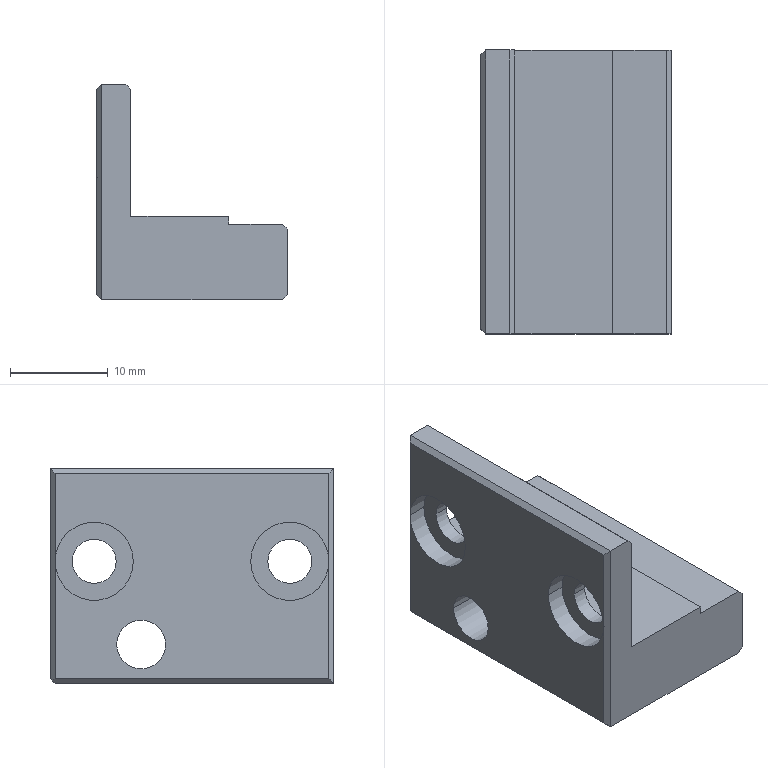Part | NX | 1 solid | 30 faces | box 19.5 x 29 x 22 mm | volume 5380 mm3 | plane 20 | cylinder 10 | commonest cylinder face diameters 4.5 x4 8 x4 5 x2
STEP:
#1=CARTESIAN_POINT('',(14.,3.2,-9.8));
#2=VERTEX_POINT('',#1);
#3=CARTESIAN_POINT('',(14.,32.2,-9.8));
#4=VERTEX_POINT('',#3);
#5=CARTESIAN_POINT('',(14.,0.,-9.8));
#6=DIRECTION('',(0.,1.,0.));
#7=VECTOR('',#6,1000.);
#8=LINE('',#5,#7);
#9=EDGE_CURVE('',#2,#4,#8,.T.);
#10=ORIENTED_EDGE('',*,*,#9,.F.);
#11=CARTESIAN_POINT('',(19.5,3.2,-9.8));
#12=VERTEX_POINT('',#11);
#13=CARTESIAN_POINT('',(0.,3.2,-9.8));
#14=DIRECTION('',(-1.,0.,0.));
#15=VECTOR('',#14,1000.);
#16=LINE('',#13,#15);
#17=EDGE_CURVE('',#12,#2,#16,.T.);
#18=ORIENTED_EDGE('',*,*,#17,.F.);
#19=CARTESIAN_POINT('',(19.5,32.2,-9.8));
#20=VERTEX_POINT('',#19);
#21=CARTESIAN_POINT('',(19.5,0.,-9.8));
#22=DIRECTION('',(0.,1.,0.));
#23=VECTOR('',#22,1000.);
#24=LINE('',#21,#23);
#25=EDGE_CURVE('',#12,#20,#24,.T.);
#26=ORIENTED_EDGE('',*,*,#25,.T.);
#27=CARTESIAN_POINT('',(0.,32.2,-9.8));
#28=DIRECTION('',(1.,0.,0.));
#29=VECTOR('',#28,1000.);
#30=LINE('',#27,#29);
#31=EDGE_CURVE('',#4,#20,#30,.T.);
#32=ORIENTED_EDGE('',*,*,#31,.F.);
#33=EDGE_LOOP('',(#10,#18,#26,#32));
#34=FACE_BOUND('',#33,.T.);
#35=CARTESIAN_POINT('',(14.,14.5,-9.8));
#36=DIRECTION('',(0.,0.,1.));
#37=DIRECTION('',(1.,0.,0.));
#38=AXIS2_PLACEMENT_3D('',#35,#36,#37);
#39=PLANE('',#38);
#40=ADVANCED_FACE('',(#34),#39,.T.);
#41=CARTESIAN_POINT('',(20.,32.2,-10.3));
#42=VERTEX_POINT('',#41);
#43=CARTESIAN_POINT('',(20.,3.2,-10.3));
#44=VERTEX_POINT('',#43);
#45=CARTESIAN_POINT('',(20.,0.,-10.3));
#46=DIRECTION('',(0.,-1.,0.));
#47=VECTOR('',#46,1000.);
#48=LINE('',#45,#47);
#49=EDGE_CURVE('',#42,#44,#48,.T.);
#50=ORIENTED_EDGE('',*,*,#49,.T.);
#51=CARTESIAN_POINT('',(20.,3.2,-17.));
#52=VERTEX_POINT('',#51);
#53=CARTESIAN_POINT('',(20.,3.2,0.));
#54=DIRECTION('',(0.,0.,1.));
#55=VECTOR('',#54,1000.);
#56=LINE('',#53,#55);
#57=EDGE_CURVE('',#52,#44,#56,.T.);
#58=ORIENTED_EDGE('',*,*,#57,.F.);
#59=CARTESIAN_POINT('',(20.,32.2,-17.));
#60=VERTEX_POINT('',#59);
#61=CARTESIAN_POINT('',(20.,0.,-17.));
#62=DIRECTION('',(0.,-1.,0.));
#63=VECTOR('',#62,1000.);
#64=LINE('',#61,#63);
#65=EDGE_CURVE('',#60,#52,#64,.T.);
#66=ORIENTED_EDGE('',*,*,#65,.F.);
#67=CARTESIAN_POINT('',(20.,32.2,0.));
#68=DIRECTION('',(0.,0.,1.));
#69=VECTOR('',#68,1000.);
#70=LINE('',#67,#69);
#71=EDGE_CURVE('',#60,#42,#70,.T.);
#72=ORIENTED_EDGE('',*,*,#71,.T.);
#73=EDGE_LOOP('',(#50,#58,#66,#72));
#74=FACE_BOUND('',#73,.T.);
#75=CARTESIAN_POINT('',(20.,25.4,-13.5));
#76=VERTEX_POINT('',#75);
#77=CARTESIAN_POINT('',(20.,20.4,-13.5));
#78=VERTEX_POINT('',#77);
#79=CARTESIAN_POINT('',(20.,22.9,-13.5));
#80=DIRECTION('',(1.,0.,0.));
#81=DIRECTION('',(0.,1.,0.));
#82=AXIS2_PLACEMENT_3D('',#79,#80,#81);
#83=CIRCLE('',#82,2.5);
#84=EDGE_CURVE('',#76,#78,#83,.T.);
#85=ORIENTED_EDGE('',*,*,#84,.F.);
#86=CARTESIAN_POINT('',(20.,22.9,-13.5));
#87=DIRECTION('',(1.,0.,0.));
#88=DIRECTION('',(0.,1.,0.));
#89=AXIS2_PLACEMENT_3D('',#86,#87,#88);
#90=CIRCLE('',#89,2.5);
#91=EDGE_CURVE('',#78,#76,#90,.T.);
#92=ORIENTED_EDGE('',*,*,#91,.F.);
#93=EDGE_LOOP('',(#85,#92));
#94=FACE_BOUND('',#93,.T.);
#95=CARTESIAN_POINT('',(20.,14.5,-10.3));
#96=DIRECTION('',(1.,0.,0.));
#97=DIRECTION('',(0.,1.,0.));
#98=AXIS2_PLACEMENT_3D('',#95,#96,#97);
#99=PLANE('',#98);
#100=ADVANCED_FACE('',(#74,#94),#99,.T.);
#101=CARTESIAN_POINT('',(1.,3.2,4.5));
#102=VERTEX_POINT('',#101);
#103=CARTESIAN_POINT('',(1.,3.2,-17.5));
#104=VERTEX_POINT('',#103);
#105=CARTESIAN_POINT('',(1.,3.2,0.));
#106=DIRECTION('',(0.,0.,-1.));
#107=VECTOR('',#106,1000.);
#108=LINE('',#105,#107);
#109=EDGE_CURVE('',#102,#104,#108,.T.);
#110=ORIENTED_EDGE('',*,*,#109,.F.);
#111=CARTESIAN_POINT('',(0.5,3.7,4.));
#112=VERTEX_POINT('',#111);
#113=CARTESIAN_POINT('',(-3.5,7.7,0.));
#114=DIRECTION('',(0.5774,-0.5774,0.5774));
#115=VECTOR('',#114,1000.);
#116=LINE('',#113,#115);
#117=EDGE_CURVE('',#112,#102,#116,.T.);
#118=ORIENTED_EDGE('',*,*,#117,.F.);
#119=CARTESIAN_POINT('',(0.5,3.7,-5.));
#120=VERTEX_POINT('',#119);
#121=CARTESIAN_POINT('',(0.5,3.7,0.));
#122=DIRECTION('',(0.,0.,1.));
#123=VECTOR('',#122,1000.);
#124=LINE('',#121,#123);
#125=EDGE_CURVE('',#120,#112,#124,.T.);
#126=ORIENTED_EDGE('',*,*,#125,.F.);
#127=CARTESIAN_POINT('',(0.5,3.7,-17.));
#128=VERTEX_POINT('',#127);
#129=CARTESIAN_POINT('',(0.5,3.7,0.));
#130=DIRECTION('',(0.,0.,1.));
#131=VECTOR('',#130,1000.);
#132=LINE('',#129,#131);
#133=EDGE_CURVE('',#128,#120,#132,.T.);
#134=ORIENTED_EDGE('',*,*,#133,.F.);
#135=CARTESIAN_POINT('',(-16.5,20.7,0.));
#136=DIRECTION('',(-0.5774,0.5774,0.5774));
#137=VECTOR('',#136,1000.);
#138=LINE('',#135,#137);
#139=EDGE_CURVE('',#104,#128,#138,.T.);
#140=ORIENTED_EDGE('',*,*,#139,.F.);
#141=EDGE_LOOP('',(#110,#118,#126,#134,#140));
#142=FACE_BOUND('',#141,.T.);
#143=CARTESIAN_POINT('',(0.75,3.45,-6.5));
#144=DIRECTION('',(0.7071,0.7071,0.));
#145=DIRECTION('',(0.,0.,-1.));
#146=AXIS2_PLACEMENT_3D('',#143,#144,#145);
#147=PLANE('',#146);
#148=ADVANCED_FACE('',(#142),#147,.F.);
#149=CARTESIAN_POINT('',(14.,32.2,-9.));
#150=VERTEX_POINT('',#149);
#151=CARTESIAN_POINT('',(14.,3.2,-9.));
#152=VERTEX_POINT('',#151);
#153=CARTESIAN_POINT('',(14.,0.,-9.));
#154=DIRECTION('',(0.,-1.,0.));
#155=VECTOR('',#154,1000.);
#156=LINE('',#153,#155);
#157=EDGE_CURVE('',#150,#152,#156,.T.);
#158=ORIENTED_EDGE('',*,*,#157,.F.);
#159=CARTESIAN_POINT('',(4.,32.2,-9.));
#160=VERTEX_POINT('',#159);
#161=CARTESIAN_POINT('',(0.,32.2,-9.));
#162=DIRECTION('',(-1.,0.,0.));
#163=VECTOR('',#162,1000.);
#164=LINE('',#161,#163);
#165=EDGE_CURVE('',#150,#160,#164,.T.);
#166=ORIENTED_EDGE('',*,*,#165,.T.);
#167=CARTESIAN_POINT('',(4.,3.2,-9.));
#168=VERTEX_POINT('',#167);
#169=CARTESIAN_POINT('',(4.,0.,-9.));
#170=DIRECTION('',(0.,1.,0.));
#171=VECTOR('',#170,1000.);
#172=LINE('',#169,#171);
#173=EDGE_CURVE('',#168,#160,#172,.T.);
#174=ORIENTED_EDGE('',*,*,#173,.F.);
#175=CARTESIAN_POINT('',(0.,3.2,-9.));
#176=DIRECTION('',(-1.,0.,0.));
#177=VECTOR('',#176,1000.);
#178=LINE('',#175,#177);
#179=EDGE_CURVE('',#152,#168,#178,.T.);
#180=ORIENTED_EDGE('',*,*,#179,.F.);
#181=EDGE_LOOP('',(#158,#166,#174,#180));
#182=FACE_BOUND('',#181,.T.);
#183=CARTESIAN_POINT('',(4.,0.,-9.));
#184=DIRECTION('',(0.,0.,1.));
#185=DIRECTION('',(1.,0.,0.));
#186=AXIS2_PLACEMENT_3D('',#183,#184,#185);
#187=PLANE('',#186);
#188=ADVANCED_FACE('',(#182),#187,.T.);
#189=ORIENTED_EDGE('',*,*,#109,.T.);
#190=CARTESIAN_POINT('',(19.5,3.2,-17.5));
#191=VERTEX_POINT('',#190);
#192=CARTESIAN_POINT('',(0.,3.2,-17.5));
#193=DIRECTION('',(1.,0.,0.));
#194=VECTOR('',#193,1000.);
#195=LINE('',#192,#194);
#196=EDGE_CURVE('',#104,#191,#195,.T.);
#197=ORIENTED_EDGE('',*,*,#196,.T.);
#198=CARTESIAN_POINT('',(37.,3.2,0.));
#199=DIRECTION('',(0.7071,0.,0.7071));
#200=VECTOR('',#199,1000.);
#201=LINE('',#198,#200);
#202=EDGE_CURVE('',#191,#52,#201,.T.);
#203=ORIENTED_EDGE('',*,*,#202,.T.);
#204=ORIENTED_EDGE('',*,*,#57,.T.);
#205=CARTESIAN_POINT('',(9.7,3.2,0.));
#206=DIRECTION('',(-0.7071,0.,0.7071));
#207=VECTOR('',#206,1000.);
#208=LINE('',#205,#207);
#209=EDGE_CURVE('',#44,#12,#208,.T.);
#210=ORIENTED_EDGE('',*,*,#209,.T.);
#211=ORIENTED_EDGE('',*,*,#17,.T.);
#212=CARTESIAN_POINT('',(14.,3.2,0.));
#213=DIRECTION('',(0.,0.,-1.));
#214=VECTOR('',#213,1000.);
#215=LINE('',#212,#214);
#216=EDGE_CURVE('',#152,#2,#215,.T.);
#217=ORIENTED_EDGE('',*,*,#216,.F.);
#218=ORIENTED_EDGE('',*,*,#179,.T.);
#219=CARTESIAN_POINT('',(4.,3.2,4.));
#220=VERTEX_POINT('',#219);
#221=CARTESIAN_POINT('',(4.,3.2,0.));
#222=DIRECTION('',(0.,0.,1.));
#223=VECTOR('',#222,1000.);
#224=LINE('',#221,#223);
#225=EDGE_CURVE('',#168,#220,#224,.T.);
#226=ORIENTED_EDGE('',*,*,#225,.T.);
#227=CARTESIAN_POINT('',(3.5,3.2,4.5));
#228=VERTEX_POINT('',#227);
#229=CARTESIAN_POINT('',(8.,3.2,0.));
#230=DIRECTION('',(0.7071,0.,-0.7071));
#231=VECTOR('',#230,1000.);
#232=LINE('',#229,#231);
#233=EDGE_CURVE('',#228,#220,#232,.T.);
#234=ORIENTED_EDGE('',*,*,#233,.F.);
#235=CARTESIAN_POINT('',(0.,3.2,4.5));
#236=DIRECTION('',(-1.,0.,0.));
#237=VECTOR('',#236,1000.);
#238=LINE('',#235,#237);
#239=EDGE_CURVE('',#228,#102,#238,.T.);
#240=ORIENTED_EDGE('',*,*,#239,.T.);
#241=EDGE_LOOP('',(#189,#197,#203,#204,#210,#211,#217,#218,#226,#234,#240));
#242=FACE_BOUND('',#241,.T.);
#243=CARTESIAN_POINT('',(17.967,3.2,-12.374));
#244=DIRECTION('',(0.,-1.,0.));
#245=DIRECTION('',(0.,0.,-1.));
#246=AXIS2_PLACEMENT_3D('',#243,#244,#245);
#247=PLANE('',#246);
#248=ADVANCED_FACE('',(#242),#247,.T.);
#249=CARTESIAN_POINT('',(1.,32.2,4.5));
#250=VERTEX_POINT('',#249);
#251=CARTESIAN_POINT('',(1.,0.,4.5));
#252=DIRECTION('',(0.,-1.,0.));
#253=VECTOR('',#252,1000.);
#254=LINE('',#251,#253);
#255=EDGE_CURVE('',#250,#102,#254,.T.);
#256=ORIENTED_EDGE('',*,*,#255,.T.);
#257=ORIENTED_EDGE('',*,*,#239,.F.);
#258=CARTESIAN_POINT('',(3.5,32.2,4.5));
#259=VERTEX_POINT('',#258);
#260=CARTESIAN_POINT('',(3.5,0.,4.5));
#261=DIRECTION('',(0.,-1.,0.));
#262=VECTOR('',#261,1000.);
#263=LINE('',#260,#262);
#264=EDGE_CURVE('',#259,#228,#263,.T.);
#265=ORIENTED_EDGE('',*,*,#264,.F.);
#266=CARTESIAN_POINT('',(0.,32.2,4.5));
#267=DIRECTION('',(-1.,0.,0.));
#268=VECTOR('',#267,1000.);
#269=LINE('',#266,#268);
#270=EDGE_CURVE('',#259,#250,#269,.T.);
#271=ORIENTED_EDGE('',*,*,#270,.T.);
#272=EDGE_LOOP('',(#256,#257,#265,#271));
#273=FACE_BOUND('',#272,.T.);
#274=CARTESIAN_POINT('',(0.,0.,4.5));
#275=DIRECTION('',(0.,0.,1.));
#276=DIRECTION('',(1.,0.,0.));
#277=AXIS2_PLACEMENT_3D('',#274,#275,#276);
#278=PLANE('',#277);
#279=ADVANCED_FACE('',(#273),#278,.T.);
#280=CARTESIAN_POINT('',(2.5,11.7,-5.));
#281=VERTEX_POINT('',#280);
#282=CARTESIAN_POINT('',(2.5,3.7,-5.));
#283=VERTEX_POINT('',#282);
#284=CARTESIAN_POINT('',(2.5,7.7,-5.));
#285=DIRECTION('',(-1.,0.,0.));
#286=DIRECTION('',(0.,1.,0.));
#287=AXIS2_PLACEMENT_3D('',#284,#285,#286);
#288=CIRCLE('',#287,4.);
#289=EDGE_CURVE('',#281,#283,#288,.T.);
#290=ORIENTED_EDGE('',*,*,#289,.T.);
#291=CARTESIAN_POINT('',(2.5,7.7,-5.));
#292=DIRECTION('',(-1.,0.,0.));
#293=DIRECTION('',(0.,1.,0.));
#294=AXIS2_PLACEMENT_3D('',#291,#292,#293);
#295=CIRCLE('',#294,4.);
#296=EDGE_CURVE('',#283,#281,#295,.T.);
#297=ORIENTED_EDGE('',*,*,#296,.T.);
#298=EDGE_LOOP('',(#290,#297));
#299=FACE_BOUND('',#298,.T.);
#300=CARTESIAN_POINT('',(2.5,5.45,-5.));
#301=VERTEX_POINT('',#300);
#302=CARTESIAN_POINT('',(2.5,9.95,-5.));
#303=VERTEX_POINT('',#302);
#304=CARTESIAN_POINT('',(2.5,7.7,-5.));
#305=DIRECTION('',(-1.,0.,0.));
#306=DIRECTION('',(0.,1.,0.));
#307=AXIS2_PLACEMENT_3D('',#304,#305,#306);
#308=CIRCLE('',#307,2.25);
#309=EDGE_CURVE('',#301,#303,#308,.T.);
#310=ORIENTED_EDGE('',*,*,#309,.F.);
#311=CARTESIAN_POINT('',(2.5,7.7,-5.));
#312=DIRECTION('',(-1.,0.,0.));
#313=DIRECTION('',(0.,1.,0.));
#314=AXIS2_PLACEMENT_3D('',#311,#312,#313);
#315=CIRCLE('',#314,2.25);
#316=EDGE_CURVE('',#303,#301,#315,.T.);
#317=ORIENTED_EDGE('',*,*,#316,.F.);
#318=EDGE_LOOP('',(#310,#317));
#319=FACE_BOUND('',#318,.T.);
#320=CARTESIAN_POINT('',(2.5,7.7,-5.));
#321=DIRECTION('',(-1.,0.,0.));
#322=DIRECTION('',(0.,0.,1.));
#323=AXIS2_PLACEMENT_3D('',#320,#321,#322);
#324=PLANE('',#323);
#325=ADVANCED_FACE('',(#299,#319),#324,.T.);
#326=CARTESIAN_POINT('',(1.,32.2,-17.));
#327=VERTEX_POINT('',#326);
#328=CARTESIAN_POINT('',(0.,32.2,-17.));
#329=DIRECTION('',(-1.,0.,0.));
#330=VECTOR('',#329,1000.);
#331=LINE('',#328,#330);
#332=EDGE_CURVE('',#60,#327,#331,.T.);
#333=ORIENTED_EDGE('',*,*,#332,.T.);
#334=CARTESIAN_POINT('',(1.,32.2,0.));
#335=DIRECTION('',(0.,0.,-1.));
#336=VECTOR('',#335,1000.);
#337=LINE('',#334,#336);
#338=EDGE_CURVE('',#250,#327,#337,.T.);
#339=ORIENTED_EDGE('',*,*,#338,.F.);
#340=ORIENTED_EDGE('',*,*,#270,.F.);
#341=CARTESIAN_POINT('',(4.,32.2,4.));
#342=VERTEX_POINT('',#341);
#343=CARTESIAN_POINT('',(8.,32.2,0.));
#344=DIRECTION('',(0.7071,0.,-0.7071));
#345=VECTOR('',#344,1000.);
#346=LINE('',#343,#345);
#347=EDGE_CURVE('',#259,#342,#346,.T.);
#348=ORIENTED_EDGE('',*,*,#347,.T.);
#349=CARTESIAN_POINT('',(4.,32.2,0.));
#350=DIRECTION('',(0.,0.,-1.));
#351=VECTOR('',#350,1000.);
#352=LINE('',#349,#351);
#353=EDGE_CURVE('',#342,#160,#352,.T.);
#354=ORIENTED_EDGE('',*,*,#353,.T.);
#355=ORIENTED_EDGE('',*,*,#165,.F.);
#356=CARTESIAN_POINT('',(14.,32.2,0.));
#357=DIRECTION('',(0.,0.,-1.));
#358=VECTOR('',#357,1000.);
#359=LINE('',#356,#358);
#360=EDGE_CURVE('',#150,#4,#359,.T.);
#361=ORIENTED_EDGE('',*,*,#360,.T.);
#362=ORIENTED_EDGE('',*,*,#31,.T.);
#363=CARTESIAN_POINT('',(9.7,32.2,0.));
#364=DIRECTION('',(0.7071,0.,-0.7071));
#365=VECTOR('',#364,1000.);
#366=LINE('',#363,#365);
#367=EDGE_CURVE('',#20,#42,#366,.T.);
#368=ORIENTED_EDGE('',*,*,#367,.T.);
#369=ORIENTED_EDGE('',*,*,#71,.F.);
#370=EDGE_LOOP('',(#333,#339,#340,#348,#354,#355,#361,#362,#368,#369));
#371=FACE_BOUND('',#370,.T.);
#372=CARTESIAN_POINT('',(0.,32.2,0.));
#373=DIRECTION('',(0.,1.,0.));
#374=DIRECTION('',(1.,0.,0.));
#375=AXIS2_PLACEMENT_3D('',#372,#373,#374);
#376=PLANE('',#375);
#377=ADVANCED_FACE('',(#371),#376,.T.);
#378=CARTESIAN_POINT('',(0.5,31.7,4.));
#379=VERTEX_POINT('',#378);
#380=CARTESIAN_POINT('',(0.5,0.,4.));
#381=DIRECTION('',(0.,-1.,0.));
#382=VECTOR('',#381,1000.);
#383=LINE('',#380,#382);
#384=EDGE_CURVE('',#379,#112,#383,.T.);
#385=ORIENTED_EDGE('',*,*,#384,.F.);
#386=CARTESIAN_POINT('',(0.5,31.7,-5.));
#387=VERTEX_POINT('',#386);
#388=CARTESIAN_POINT('',(0.5,31.7,0.));
#389=DIRECTION('',(0.,0.,1.));
#390=VECTOR('',#389,1000.);
#391=LINE('',#388,#390);
#392=EDGE_CURVE('',#387,#379,#391,.T.);
#393=ORIENTED_EDGE('',*,*,#392,.F.);
#394=CARTESIAN_POINT('',(0.5,23.7,-5.));
#395=VERTEX_POINT('',#394);
#396=CARTESIAN_POINT('',(0.5,27.7,-5.));
#397=DIRECTION('',(-1.,0.,0.));
#398=DIRECTION('',(0.,1.,0.));
#399=AXIS2_PLACEMENT_3D('',#396,#397,#398);
#400=CIRCLE('',#399,4.);
#401=EDGE_CURVE('',#395,#387,#400,.T.);
#402=ORIENTED_EDGE('',*,*,#401,.F.);
#403=CARTESIAN_POINT('',(0.5,27.7,-5.));
#404=DIRECTION('',(-1.,0.,0.));
#405=DIRECTION('',(0.,1.,0.));
#406=AXIS2_PLACEMENT_3D('',#403,#404,#405);
#407=CIRCLE('',#406,4.);
#408=EDGE_CURVE('',#387,#395,#407,.T.);
#409=ORIENTED_EDGE('',*,*,#408,.F.);
#410=CARTESIAN_POINT('',(0.5,31.7,-17.));
#411=VERTEX_POINT('',#410);
#412=CARTESIAN_POINT('',(0.5,31.7,0.));
#413=DIRECTION('',(0.,0.,1.));
#414=VECTOR('',#413,1000.);
#415=LINE('',#412,#414);
#416=EDGE_CURVE('',#411,#387,#415,.T.);
#417=ORIENTED_EDGE('',*,*,#416,.F.);
#418=CARTESIAN_POINT('',(0.5,0.,-17.));
#419=DIRECTION('',(0.,1.,0.));
#420=VECTOR('',#419,1000.);
#421=LINE('',#418,#420);
#422=EDGE_CURVE('',#128,#411,#421,.T.);
#423=ORIENTED_EDGE('',*,*,#422,.F.);
#424=ORIENTED_EDGE('',*,*,#133,.T.);
#425=CARTESIAN_POINT('',(0.5,11.7,-5.));
#426=VERTEX_POINT('',#425);
#427=CARTESIAN_POINT('',(0.5,7.7,-5.));
#428=DIRECTION('',(-1.,0.,0.));
#429=DIRECTION('',(0.,1.,0.));
#430=AXIS2_PLACEMENT_3D('',#427,#428,#429);
#431=CIRCLE('',#430,4.);
#432=EDGE_CURVE('',#426,#120,#431,.T.);
#433=ORIENTED_EDGE('',*,*,#432,.F.);
#434=CARTESIAN_POINT('',(0.5,7.7,-5.));
#435=DIRECTION('',(-1.,0.,0.));
#436=DIRECTION('',(0.,1.,0.));
#437=AXIS2_PLACEMENT_3D('',#434,#435,#436);
#438=CIRCLE('',#437,4.);
#439=EDGE_CURVE('',#120,#426,#438,.T.);
#440=ORIENTED_EDGE('',*,*,#439,.F.);
#441=ORIENTED_EDGE('',*,*,#125,.T.);
#442=EDGE_LOOP('',(#385,#393,#402,#409,#417,#423,#424,#433,#440,#441));
#443=FACE_BOUND('',#442,.T.);
#444=CARTESIAN_POINT('',(0.5,25.4,-13.5));
#445=VERTEX_POINT('',#444);
#446=CARTESIAN_POINT('',(0.5,20.4,-13.5));
#447=VERTEX_POINT('',#446);
#448=CARTESIAN_POINT('',(0.5,22.9,-13.5));
#449=DIRECTION('',(1.,0.,0.));
#450=DIRECTION('',(0.,1.,0.));
#451=AXIS2_PLACEMENT_3D('',#448,#449,#450);
#452=CIRCLE('',#451,2.5);
#453=EDGE_CURVE('',#445,#447,#452,.T.);
#454=ORIENTED_EDGE('',*,*,#453,.T.);
#455=CARTESIAN_POINT('',(0.5,22.9,-13.5));
#456=DIRECTION('',(1.,0.,0.));
#457=DIRECTION('',(0.,1.,0.));
#458=AXIS2_PLACEMENT_3D('',#455,#456,#457);
#459=CIRCLE('',#458,2.5);
#460=EDGE_CURVE('',#447,#445,#459,.T.);
#461=ORIENTED_EDGE('',*,*,#460,.T.);
#462=EDGE_LOOP('',(#454,#461));
#463=FACE_BOUND('',#462,.T.);
#464=CARTESIAN_POINT('',(0.5,14.5,-17.));
#465=DIRECTION('',(-1.,0.,0.));
#466=DIRECTION('',(0.,0.,1.));
#467=AXIS2_PLACEMENT_3D('',#464,#465,#466);
#468=PLANE('',#467);
#469=ADVANCED_FACE('',(#443,#463),#468,.T.);
#470=ORIENTED_EDGE('',*,*,#117,.T.);
#471=ORIENTED_EDGE('',*,*,#255,.F.);
#472=CARTESIAN_POINT('',(-3.5,27.7,0.));
#473=DIRECTION('',(0.5774,0.5774,0.5774));
#474=VECTOR('',#473,1000.);
#475=LINE('',#472,#474);
#476=EDGE_CURVE('',#379,#250,#475,.T.);
#477=ORIENTED_EDGE('',*,*,#476,.F.);
#478=ORIENTED_EDGE('',*,*,#384,.T.);
#479=EDGE_LOOP('',(#470,#471,#477,#478));
#480=FACE_BOUND('',#479,.T.);
#481=CARTESIAN_POINT('',(0.75,17.,4.25));
#482=DIRECTION('',(-0.7071,0.,0.7071));
#483=DIRECTION('',(0.,1.,0.));
#484=AXIS2_PLACEMENT_3D('',#481,#482,#483);
#485=PLANE('',#484);
#486=ADVANCED_FACE('',(#480),#485,.T.);
#487=ORIENTED_EDGE('',*,*,#453,.F.);
#488=CARTESIAN_POINT('',(0.,25.4,-13.5));
#489=DIRECTION('',(1.,0.,0.));
#490=VECTOR('',#489,1000.);
#491=LINE('',#488,#490);
#492=EDGE_CURVE('',#445,#76,#491,.T.);
#493=ORIENTED_EDGE('',*,*,#492,.T.);
#494=ORIENTED_EDGE('',*,*,#84,.T.);
#495=CARTESIAN_POINT('',(0.,20.4,-13.5));
#496=DIRECTION('',(1.,0.,0.));
#497=VECTOR('',#496,1000.);
#498=LINE('',#495,#497);
#499=EDGE_CURVE('',#447,#78,#498,.T.);
#500=ORIENTED_EDGE('',*,*,#499,.F.);
#501=EDGE_LOOP('',(#487,#493,#494,#500));
#502=FACE_BOUND('',#501,.T.);
#503=CARTESIAN_POINT('',(0.,22.9,-13.5));
#504=DIRECTION('',(1.,0.,0.));
#505=DIRECTION('',(0.,1.,0.));
#506=AXIS2_PLACEMENT_3D('',#503,#504,#505);
#507=CYLINDRICAL_SURFACE('',#506,2.5);
#508=ADVANCED_FACE('',(#502),#507,.F.);
#509=CARTESIAN_POINT('',(2.5,31.7,-5.));
#510=VERTEX_POINT('',#509);
#511=CARTESIAN_POINT('',(2.5,23.7,-5.));
#512=VERTEX_POINT('',#511);
#513=CARTESIAN_POINT('',(2.5,27.7,-5.));
#514=DIRECTION('',(-1.,0.,0.));
#515=DIRECTION('',(0.,1.,0.));
#516=AXIS2_PLACEMENT_3D('',#513,#514,#515);
#517=CIRCLE('',#516,4.);
#518=EDGE_CURVE('',#510,#512,#517,.T.);
#519=ORIENTED_EDGE('',*,*,#518,.T.);
#520=CARTESIAN_POINT('',(2.5,27.7,-5.));
#521=DIRECTION('',(-1.,0.,0.));
#522=DIRECTION('',(0.,1.,0.));
#523=AXIS2_PLACEMENT_3D('',#520,#521,#522);
#524=CIRCLE('',#523,4.);
#525=EDGE_CURVE('',#512,#510,#524,.T.);
#526=ORIENTED_EDGE('',*,*,#525,.T.);
#527=EDGE_LOOP('',(#519,#526));
#528=FACE_BOUND('',#527,.T.);
#529=CARTESIAN_POINT('',(2.5,29.95,-5.));
#530=VERTEX_POINT('',#529);
#531=CARTESIAN_POINT('',(2.5,25.45,-5.));
#532=VERTEX_POINT('',#531);
#533=CARTESIAN_POINT('',(2.5,27.7,-5.));
#534=DIRECTION('',(-1.,0.,0.));
#535=DIRECTION('',(0.,1.,0.));
#536=AXIS2_PLACEMENT_3D('',#533,#534,#535);
#537=CIRCLE('',#536,2.25);
#538=EDGE_CURVE('',#530,#532,#537,.T.);
#539=ORIENTED_EDGE('',*,*,#538,.F.);
#540=CARTESIAN_POINT('',(2.5,27.7,-5.));
#541=DIRECTION('',(-1.,0.,0.));
#542=DIRECTION('',(0.,1.,0.));
#543=AXIS2_PLACEMENT_3D('',#540,#541,#542);
#544=CIRCLE('',#543,2.25);
#545=EDGE_CURVE('',#532,#530,#544,.T.);
#546=ORIENTED_EDGE('',*,*,#545,.F.);
#547=EDGE_LOOP('',(#539,#546));
#548=FACE_BOUND('',#547,.T.);
#549=CARTESIAN_POINT('',(2.5,27.7,-5.));
#550=DIRECTION('',(-1.,0.,0.));
#551=DIRECTION('',(0.,0.,1.));
#552=AXIS2_PLACEMENT_3D('',#549,#550,#551);
#553=PLANE('',#552);
#554=ADVANCED_FACE('',(#528,#548),#553,.T.);
#555=ORIENTED_EDGE('',*,*,#432,.T.);
#556=CARTESIAN_POINT('',(23.1,3.7,-5.));
#557=DIRECTION('',(-1.,0.,0.));
#558=VECTOR('',#557,1000.);
#559=LINE('',#556,#558);
#560=EDGE_CURVE('',#283,#120,#559,.T.);
#561=ORIENTED_EDGE('',*,*,#560,.F.);
#562=ORIENTED_EDGE('',*,*,#289,.F.);
#563=CARTESIAN_POINT('',(23.1,11.7,-5.));
#564=DIRECTION('',(-1.,0.,0.));
#565=VECTOR('',#564,1000.);
#566=LINE('',#563,#565);
#567=EDGE_CURVE('',#281,#426,#566,.T.);
#568=ORIENTED_EDGE('',*,*,#567,.T.);
#569=EDGE_LOOP('',(#555,#561,#562,#568));
#570=FACE_BOUND('',#569,.T.);
#571=CARTESIAN_POINT('',(23.1,7.7,-5.));
#572=DIRECTION('',(-1.,0.,0.));
#573=DIRECTION('',(0.,1.,0.));
#574=AXIS2_PLACEMENT_3D('',#571,#572,#573);
#575=CYLINDRICAL_SURFACE('',#574,4.);
#576=ADVANCED_FACE('',(#570),#575,.F.);
#577=ORIENTED_EDGE('',*,*,#538,.T.);
#578=CARTESIAN_POINT('',(4.,25.45,-5.));
#579=VERTEX_POINT('',#578);
#580=CARTESIAN_POINT('',(23.1,25.45,-5.));
#581=DIRECTION('',(-1.,0.,0.));
#582=VECTOR('',#581,1000.);
#583=LINE('',#580,#582);
#584=EDGE_CURVE('',#579,#532,#583,.T.);
#585=ORIENTED_EDGE('',*,*,#584,.F.);
#586=CARTESIAN_POINT('',(4.,29.95,-5.));
#587=VERTEX_POINT('',#586);
#588=CARTESIAN_POINT('',(4.,27.7,-5.));
#589=DIRECTION('',(-1.,0.,0.));
#590=DIRECTION('',(0.,1.,0.));
#591=AXIS2_PLACEMENT_3D('',#588,#589,#590);
#592=CIRCLE('',#591,2.25);
#593=EDGE_CURVE('',#587,#579,#592,.T.);
#594=ORIENTED_EDGE('',*,*,#593,.F.);
#595=CARTESIAN_POINT('',(23.1,29.95,-5.));
#596=DIRECTION('',(-1.,0.,0.));
#597=VECTOR('',#596,1000.);
#598=LINE('',#595,#597);
#599=EDGE_CURVE('',#587,#530,#598,.T.);
#600=ORIENTED_EDGE('',*,*,#599,.T.);
#601=EDGE_LOOP('',(#577,#585,#594,#600));
#602=FACE_BOUND('',#601,.T.);
#603=CARTESIAN_POINT('',(23.1,27.7,-5.));
#604=DIRECTION('',(-1.,0.,0.));
#605=DIRECTION('',(0.,1.,0.));
#606=AXIS2_PLACEMENT_3D('',#603,#604,#605);
#607=CYLINDRICAL_SURFACE('',#606,2.25);
#608=ADVANCED_FACE('',(#602),#607,.F.);
#609=CARTESIAN_POINT('',(4.,0.,4.));
#610=DIRECTION('',(0.,-1.,0.));
#611=VECTOR('',#610,1000.);
#612=LINE('',#609,#611);
#613=EDGE_CURVE('',#342,#220,#612,.T.);
#614=ORIENTED_EDGE('',*,*,#613,.T.);
#615=ORIENTED_EDGE('',*,*,#225,.F.);
#616=ORIENTED_EDGE('',*,*,#173,.T.);
#617=ORIENTED_EDGE('',*,*,#353,.F.);
#618=EDGE_LOOP('',(#614,#615,#616,#617));
#619=FACE_BOUND('',#618,.T.);
#620=CARTESIAN_POINT('',(4.,9.95,-5.));
#621=VERTEX_POINT('',#620);
#622=CARTESIAN_POINT('',(4.,5.45,-5.));
#623=VERTEX_POINT('',#622);
#624=CARTESIAN_POINT('',(4.,7.7,-5.));
#625=DIRECTION('',(-1.,0.,0.));
#626=DIRECTION('',(0.,1.,0.));
#627=AXIS2_PLACEMENT_3D('',#624,#625,#626);
#628=CIRCLE('',#627,2.25);
#629=EDGE_CURVE('',#621,#623,#628,.T.);
#630=ORIENTED_EDGE('',*,*,#629,.T.);
#631=CARTESIAN_POINT('',(4.,7.7,-5.));
#632=DIRECTION('',(-1.,0.,0.));
#633=DIRECTION('',(0.,1.,0.));
#634=AXIS2_PLACEMENT_3D('',#631,#632,#633);
#635=CIRCLE('',#634,2.25);
#636=EDGE_CURVE('',#623,#621,#635,.T.);
#637=ORIENTED_EDGE('',*,*,#636,.T.);
#638=EDGE_LOOP('',(#630,#637));
#639=FACE_BOUND('',#638,.T.);
#640=ORIENTED_EDGE('',*,*,#593,.T.);
#641=CARTESIAN_POINT('',(4.,27.7,-5.));
#642=DIRECTION('',(-1.,0.,0.));
#643=DIRECTION('',(0.,1.,0.));
#644=AXIS2_PLACEMENT_3D('',#641,#642,#643);
#645=CIRCLE('',#644,2.25);
#646=EDGE_CURVE('',#579,#587,#645,.T.);
#647=ORIENTED_EDGE('',*,*,#646,.T.);
#648=EDGE_LOOP('',(#640,#647));
#649=FACE_BOUND('',#648,.T.);
#650=CARTESIAN_POINT('',(4.,0.,0.));
#651=DIRECTION('',(1.,0.,0.));
#652=DIRECTION('',(0.,1.,0.));
#653=AXIS2_PLACEMENT_3D('',#650,#651,#652);
#654=PLANE('',#653);
#655=ADVANCED_FACE('',(#619,#639,#649),#654,.T.);
#656=ORIENTED_EDGE('',*,*,#629,.F.);
#657=CARTESIAN_POINT('',(23.1,9.95,-5.));
#658=DIRECTION('',(-1.,0.,0.));
#659=VECTOR('',#658,1000.);
#660=LINE('',#657,#659);
#661=EDGE_CURVE('',#621,#303,#660,.T.);
#662=ORIENTED_EDGE('',*,*,#661,.T.);
#663=ORIENTED_EDGE('',*,*,#316,.T.);
#664=CARTESIAN_POINT('',(23.1,5.45,-5.));
#665=DIRECTION('',(-1.,0.,0.));
#666=VECTOR('',#665,1000.);
#667=LINE('',#664,#666);
#668=EDGE_CURVE('',#623,#301,#667,.T.);
#669=ORIENTED_EDGE('',*,*,#668,.F.);
#670=EDGE_LOOP('',(#656,#662,#663,#669));
#671=FACE_BOUND('',#670,.T.);
#672=CARTESIAN_POINT('',(23.1,7.7,-5.));
#673=DIRECTION('',(-1.,0.,0.));
#674=DIRECTION('',(0.,1.,0.));
#675=AXIS2_PLACEMENT_3D('',#672,#673,#674);
#676=CYLINDRICAL_SURFACE('',#675,2.25);
#677=ADVANCED_FACE('',(#671),#676,.F.);
#678=ORIENTED_EDGE('',*,*,#518,.F.);
#679=CARTESIAN_POINT('',(23.1,31.7,-5.));
#680=DIRECTION('',(-1.,0.,0.));
#681=VECTOR('',#680,1000.);
#682=LINE('',#679,#681);
#683=EDGE_CURVE('',#510,#387,#682,.T.);
#684=ORIENTED_EDGE('',*,*,#683,.T.);
#685=ORIENTED_EDGE('',*,*,#408,.T.);
#686=CARTESIAN_POINT('',(23.1,23.7,-5.));
#687=DIRECTION('',(-1.,0.,0.));
#688=VECTOR('',#687,1000.);
#689=LINE('',#686,#688);
#690=EDGE_CURVE('',#512,#395,#689,.T.);
#691=ORIENTED_EDGE('',*,*,#690,.F.);
#692=EDGE_LOOP('',(#678,#684,#685,#691));
#693=FACE_BOUND('',#692,.T.);
#694=CARTESIAN_POINT('',(23.1,27.7,-5.));
#695=DIRECTION('',(-1.,0.,0.));
#696=DIRECTION('',(0.,1.,0.));
#697=AXIS2_PLACEMENT_3D('',#694,#695,#696);
#698=CYLINDRICAL_SURFACE('',#697,4.);
#699=ADVANCED_FACE('',(#693),#698,.F.);
#700=CARTESIAN_POINT('',(19.5,31.7,-17.5));
#701=VERTEX_POINT('',#700);
#702=CARTESIAN_POINT('',(37.,49.2,0.));
#703=DIRECTION('',(0.5774,0.5774,0.5774));
#704=VECTOR('',#703,1000.);
#705=LINE('',#702,#704);
#706=EDGE_CURVE('',#701,#60,#705,.T.);
#707=ORIENTED_EDGE('',*,*,#706,.T.);
#708=ORIENTED_EDGE('',*,*,#65,.T.);
#709=ORIENTED_EDGE('',*,*,#202,.F.);
#710=CARTESIAN_POINT('',(19.5,0.,-17.5));
#711=DIRECTION('',(0.,1.,0.));
#712=VECTOR('',#711,1000.);
#713=LINE('',#710,#712);
#714=EDGE_CURVE('',#191,#701,#713,.T.);
#715=ORIENTED_EDGE('',*,*,#714,.T.);
#716=EDGE_LOOP('',(#707,#708,#709,#715));
#717=FACE_BOUND('',#716,.T.);
#718=CARTESIAN_POINT('',(20.,14.5,-17.));
#719=DIRECTION('',(0.7071,0.,-0.7071));
#720=DIRECTION('',(0.,-1.,0.));
#721=AXIS2_PLACEMENT_3D('',#718,#719,#720);
#722=PLANE('',#721);
#723=ADVANCED_FACE('',(#717),#722,.T.);
#724=CARTESIAN_POINT('',(1.,31.7,-17.5));
#725=VERTEX_POINT('',#724);
#726=CARTESIAN_POINT('',(1.,0.,-17.5));
#727=DIRECTION('',(0.,1.,0.));
#728=VECTOR('',#727,1000.);
#729=LINE('',#726,#728);
#730=EDGE_CURVE('',#104,#725,#729,.T.);
#731=ORIENTED_EDGE('',*,*,#730,.F.);
#732=ORIENTED_EDGE('',*,*,#139,.T.);
#733=ORIENTED_EDGE('',*,*,#422,.T.);
#734=CARTESIAN_POINT('',(0.75,31.95,-17.25));
#735=VERTEX_POINT('',#734);
#736=CARTESIAN_POINT('',(-16.5,14.7,0.));
#737=DIRECTION('',(-0.5774,-0.5774,0.5774));
#738=VECTOR('',#737,1000.);
#739=LINE('',#736,#738);
#740=EDGE_CURVE('',#735,#411,#739,.T.);
#741=ORIENTED_EDGE('',*,*,#740,.F.);
#742=CARTESIAN_POINT('',(-16.5,49.2,0.));
#743=DIRECTION('',(0.5774,-0.5774,-0.5774));
#744=VECTOR('',#743,1000.);
#745=LINE('',#742,#744);
#746=EDGE_CURVE('',#735,#725,#745,.T.);
#747=ORIENTED_EDGE('',*,*,#746,.T.);
#748=EDGE_LOOP('',(#731,#732,#733,#741,#747));
#749=FACE_BOUND('',#748,.T.);
#750=CARTESIAN_POINT('',(1.,14.5,-17.5));
#751=DIRECTION('',(-0.7071,0.,-0.7071));
#752=DIRECTION('',(-0.7071,0.,0.7071));
#753=AXIS2_PLACEMENT_3D('',#750,#751,#752);
#754=PLANE('',#753);
#755=ADVANCED_FACE('',(#749),#754,.T.);
#756=ORIENTED_EDGE('',*,*,#338,.T.);
#757=CARTESIAN_POINT('',(18.,49.2,0.));
#758=DIRECTION('',(-0.5774,-0.5774,-0.5774));
#759=VECTOR('',#758,1000.);
#760=LINE('',#757,#759);
#761=EDGE_CURVE('',#327,#735,#760,.T.);
#762=ORIENTED_EDGE('',*,*,#761,.T.);
#763=ORIENTED_EDGE('',*,*,#740,.T.);
#764=ORIENTED_EDGE('',*,*,#416,.T.);
#765=ORIENTED_EDGE('',*,*,#392,.T.);
#766=ORIENTED_EDGE('',*,*,#476,.T.);
#767=EDGE_LOOP('',(#756,#762,#763,#764,#765,#766));
#768=FACE_BOUND('',#767,.T.);
#769=CARTESIAN_POINT('',(0.75,31.95,-8.5));
#770=DIRECTION('',(-0.7071,0.7071,0.));
#771=DIRECTION('',(0.,0.,1.));
#772=AXIS2_PLACEMENT_3D('',#769,#770,#771);
#773=PLANE('',#772);
#774=ADVANCED_FACE('',(#768),#773,.T.);
#775=ORIENTED_EDGE('',*,*,#9,.T.);
#776=ORIENTED_EDGE('',*,*,#360,.F.);
#777=ORIENTED_EDGE('',*,*,#157,.T.);
#778=ORIENTED_EDGE('',*,*,#216,.T.);
#779=EDGE_LOOP('',(#775,#776,#777,#778));
#780=FACE_BOUND('',#779,.T.);
#781=CARTESIAN_POINT('',(14.,26.,-19.25));
#782=DIRECTION('',(-1.,0.,0.));
#783=DIRECTION('',(0.,0.,1.));
#784=AXIS2_PLACEMENT_3D('',#781,#782,#783);
#785=PLANE('',#784);
#786=ADVANCED_FACE('',(#780),#785,.F.);
#787=ORIENTED_EDGE('',*,*,#613,.F.);
#788=ORIENTED_EDGE('',*,*,#347,.F.);
#789=ORIENTED_EDGE('',*,*,#264,.T.);
#790=ORIENTED_EDGE('',*,*,#233,.T.);
#791=EDGE_LOOP('',(#787,#788,#789,#790));
#792=FACE_BOUND('',#791,.T.);
#793=CARTESIAN_POINT('',(3.75,17.,4.25));
#794=DIRECTION('',(-0.7071,0.,-0.7071));
#795=DIRECTION('',(-0.7071,0.,0.7071));
#796=AXIS2_PLACEMENT_3D('',#793,#794,#795);
#797=PLANE('',#796);
#798=ADVANCED_FACE('',(#792),#797,.F.);
#799=ORIENTED_EDGE('',*,*,#25,.F.);
#800=ORIENTED_EDGE('',*,*,#209,.F.);
#801=ORIENTED_EDGE('',*,*,#49,.F.);
#802=ORIENTED_EDGE('',*,*,#367,.F.);
#803=EDGE_LOOP('',(#799,#800,#801,#802));
#804=FACE_BOUND('',#803,.T.);
#805=CARTESIAN_POINT('',(19.75,19.25,-10.05));
#806=DIRECTION('',(0.7071,0.,0.7071));
#807=DIRECTION('',(0.,-1.,0.));
#808=AXIS2_PLACEMENT_3D('',#805,#806,#807);
#809=PLANE('',#808);
#810=ADVANCED_FACE('',(#804),#809,.T.);
#811=ORIENTED_EDGE('',*,*,#714,.F.);
#812=ORIENTED_EDGE('',*,*,#196,.F.);
#813=ORIENTED_EDGE('',*,*,#730,.T.);
#814=CARTESIAN_POINT('',(0.,31.7,-17.5));
#815=DIRECTION('',(1.,0.,0.));
#816=VECTOR('',#815,1000.);
#817=LINE('',#814,#816);
#818=EDGE_CURVE('',#725,#701,#817,.T.);
#819=ORIENTED_EDGE('',*,*,#818,.T.);
#820=EDGE_LOOP('',(#811,#812,#813,#819));
#821=FACE_BOUND('',#820,.T.);
#822=CARTESIAN_POINT('',(19.5,14.5,-17.5));
#823=DIRECTION('',(0.,0.,-1.));
#824=DIRECTION('',(0.,-1.,0.));
#825=AXIS2_PLACEMENT_3D('',#822,#823,#824);
#826=PLANE('',#825);
#827=ADVANCED_FACE('',(#821),#826,.T.);
#828=ORIENTED_EDGE('',*,*,#332,.F.);
#829=ORIENTED_EDGE('',*,*,#706,.F.);
#830=ORIENTED_EDGE('',*,*,#818,.F.);
#831=ORIENTED_EDGE('',*,*,#746,.F.);
#832=ORIENTED_EDGE('',*,*,#761,.F.);
#833=EDGE_LOOP('',(#828,#829,#830,#831,#832));
#834=FACE_BOUND('',#833,.T.);
#835=CARTESIAN_POINT('',(10.25,31.95,-17.25));
#836=DIRECTION('',(0.,-0.7071,0.7071));
#837=DIRECTION('',(-1.,0.,0.));
#838=AXIS2_PLACEMENT_3D('',#835,#836,#837);
#839=PLANE('',#838);
#840=ADVANCED_FACE('',(#834),#839,.F.);
#841=ORIENTED_EDGE('',*,*,#401,.T.);
#842=ORIENTED_EDGE('',*,*,#683,.F.);
#843=ORIENTED_EDGE('',*,*,#525,.F.);
#844=ORIENTED_EDGE('',*,*,#690,.T.);
#845=EDGE_LOOP('',(#841,#842,#843,#844));
#846=FACE_BOUND('',#845,.T.);
#847=CARTESIAN_POINT('',(23.1,27.7,-5.));
#848=DIRECTION('',(-1.,0.,0.));
#849=DIRECTION('',(0.,1.,0.));
#850=AXIS2_PLACEMENT_3D('',#847,#848,#849);
#851=CYLINDRICAL_SURFACE('',#850,4.);
#852=ADVANCED_FACE('',(#846),#851,.F.);
#853=ORIENTED_EDGE('',*,*,#309,.T.);
#854=ORIENTED_EDGE('',*,*,#661,.F.);
#855=ORIENTED_EDGE('',*,*,#636,.F.);
#856=ORIENTED_EDGE('',*,*,#668,.T.);
#857=EDGE_LOOP('',(#853,#854,#855,#856));
#858=FACE_BOUND('',#857,.T.);
#859=CARTESIAN_POINT('',(23.1,7.7,-5.));
#860=DIRECTION('',(-1.,0.,0.));
#861=DIRECTION('',(0.,1.,0.));
#862=AXIS2_PLACEMENT_3D('',#859,#860,#861);
#863=CYLINDRICAL_SURFACE('',#862,2.25);
#864=ADVANCED_FACE('',(#858),#863,.F.);
#865=ORIENTED_EDGE('',*,*,#492,.F.);
#866=ORIENTED_EDGE('',*,*,#460,.F.);
#867=ORIENTED_EDGE('',*,*,#499,.T.);
#868=ORIENTED_EDGE('',*,*,#91,.T.);
#869=EDGE_LOOP('',(#865,#866,#867,#868));
#870=FACE_BOUND('',#869,.T.);
#871=CARTESIAN_POINT('',(0.,22.9,-13.5));
#872=DIRECTION('',(1.,0.,0.));
#873=DIRECTION('',(0.,1.,0.));
#874=AXIS2_PLACEMENT_3D('',#871,#872,#873);
#875=CYLINDRICAL_SURFACE('',#874,2.5);
#876=ADVANCED_FACE('',(#870),#875,.F.);
#877=ORIENTED_EDGE('',*,*,#599,.F.);
#878=ORIENTED_EDGE('',*,*,#646,.F.);
#879=ORIENTED_EDGE('',*,*,#584,.T.);
#880=ORIENTED_EDGE('',*,*,#545,.T.);
#881=EDGE_LOOP('',(#877,#878,#879,#880));
#882=FACE_BOUND('',#881,.T.);
#883=CARTESIAN_POINT('',(23.1,27.7,-5.));
#884=DIRECTION('',(-1.,0.,0.));
#885=DIRECTION('',(0.,1.,0.));
#886=AXIS2_PLACEMENT_3D('',#883,#884,#885);
#887=CYLINDRICAL_SURFACE('',#886,2.25);
#888=ADVANCED_FACE('',(#882),#887,.F.);
#889=ORIENTED_EDGE('',*,*,#567,.F.);
#890=ORIENTED_EDGE('',*,*,#296,.F.);
#891=ORIENTED_EDGE('',*,*,#560,.T.);
#892=ORIENTED_EDGE('',*,*,#439,.T.);
#893=EDGE_LOOP('',(#889,#890,#891,#892));
#894=FACE_BOUND('',#893,.T.);
#895=CARTESIAN_POINT('',(23.1,7.7,-5.));
#896=DIRECTION('',(-1.,0.,0.));
#897=DIRECTION('',(0.,1.,0.));
#898=AXIS2_PLACEMENT_3D('',#895,#896,#897);
#899=CYLINDRICAL_SURFACE('',#898,4.);
#900=ADVANCED_FACE('',(#894),#899,.F.);
#901=CLOSED_SHELL('',(#40,#100,#148,#188,#248,#279,#325,#377,#469,#486,#508,#554,#576,#608,#655,#677,#699,#723,#755,#774,#786,#798,#810,#827,#840,#852,#864,#876,#888,#900));
#902=MANIFOLD_SOLID_BREP('',#901);
#903=(LENGTH_UNIT()NAMED_UNIT(*)SI_UNIT(.MILLI.,.METRE.));
#904=UNCERTAINTY_MEASURE_WITH_UNIT(LENGTH_MEASURE(0.00001),#903,'','');
#905=(NAMED_UNIT(*)PLANE_ANGLE_UNIT()SI_UNIT($,.RADIAN.));
#906=(NAMED_UNIT(*)SI_UNIT($,.STERADIAN.)SOLID_ANGLE_UNIT());
#907=(GEOMETRIC_REPRESENTATION_CONTEXT(3)GLOBAL_UNCERTAINTY_ASSIGNED_CONTEXT((#904))GLOBAL_UNIT_ASSIGNED_CONTEXT((#903,#905,#906))REPRESENTATION_CONTEXT('',''));
#908=ADVANCED_BREP_SHAPE_REPRESENTATION('',(#902),#907);